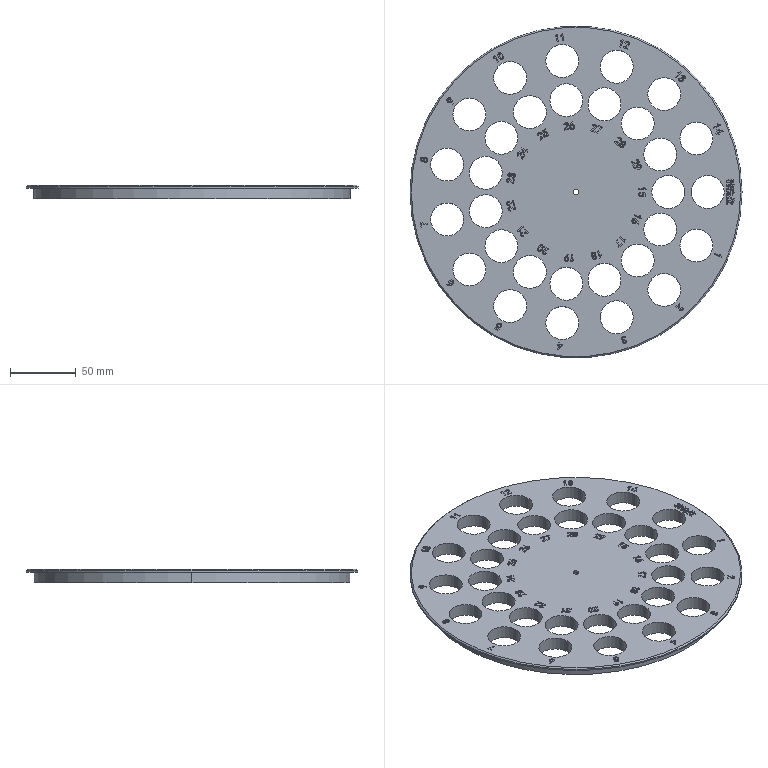Part | SolidWorks | features ICE 5, Chamfer 1, Extrusion 1, HoleWzd 1 | 1 solid | 736 faces | box 252 x 252 x 10 mm | volume 307867 mm3 | plane 419 | spline 224 | cylinder 81 | cone 12 | commonest cylinder face diameters 25 x60 3.3 x10 4.5 x2 10 x2 18.5 x2 240 x2